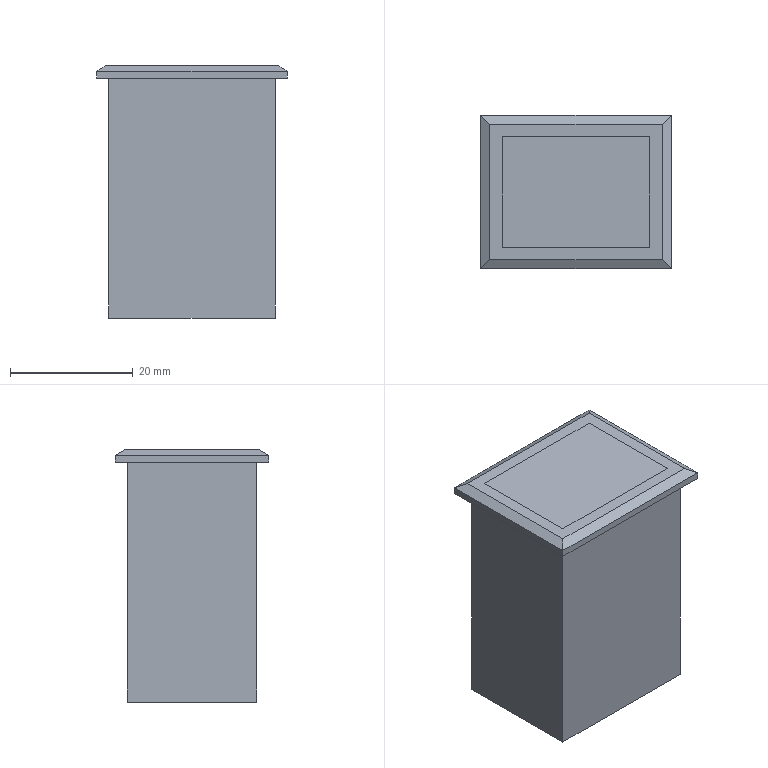Part | SolidWorks | features Chamfer 1, Extrusion 1, ICE 1, PLine 1 | 1 solid | 16 faces | box 31 x 25 x 41 mm | volume 23593 mm3 | plane 16
STEP:
#1=CARTESIAN_POINT('',(-14.,11.,41.));
#2=VERTEX_POINT('',#1);
#3=CARTESIAN_POINT('',(-14.,-11.,41.));
#4=VERTEX_POINT('',#3);
#5=CARTESIAN_POINT('',(-14.,12.5,41.));
#6=DIRECTION('',(0.,-1.,0.));
#7=VECTOR('',#6,1000.);
#8=LINE('',#5,#7);
#9=EDGE_CURVE('',#2,#4,#8,.T.);
#10=ORIENTED_EDGE('',*,*,#9,.T.);
#11=CARTESIAN_POINT('',(14.,-11.,41.));
#12=VERTEX_POINT('',#11);
#13=CARTESIAN_POINT('',(15.5,-11.,41.));
#14=DIRECTION('',(1.,0.,0.));
#15=VECTOR('',#14,1000.);
#16=LINE('',#13,#15);
#17=EDGE_CURVE('',#4,#12,#16,.T.);
#18=ORIENTED_EDGE('',*,*,#17,.T.);
#19=CARTESIAN_POINT('',(14.,11.,41.));
#20=VERTEX_POINT('',#19);
#21=CARTESIAN_POINT('',(14.,12.5,41.));
#22=DIRECTION('',(0.,1.,0.));
#23=VECTOR('',#22,1000.);
#24=LINE('',#21,#23);
#25=EDGE_CURVE('',#12,#20,#24,.T.);
#26=ORIENTED_EDGE('',*,*,#25,.T.);
#27=CARTESIAN_POINT('',(15.5,11.,41.));
#28=DIRECTION('',(-1.,0.,0.));
#29=VECTOR('',#28,1000.);
#30=LINE('',#27,#29);
#31=EDGE_CURVE('',#20,#2,#30,.T.);
#32=ORIENTED_EDGE('',*,*,#31,.T.);
#33=EDGE_LOOP('',(#10,#18,#26,#32));
#34=FACE_OUTER_BOUND('',#33,.T.);
#35=CARTESIAN_POINT('',(12.,-9.,41.));
#36=VERTEX_POINT('',#35);
#37=CARTESIAN_POINT('',(12.,9.,41.));
#38=VERTEX_POINT('',#37);
#39=CARTESIAN_POINT('',(12.,12.5,41.));
#40=DIRECTION('',(0.,1.,0.));
#41=VECTOR('',#40,1000.);
#42=LINE('',#39,#41);
#43=EDGE_CURVE('',#36,#38,#42,.T.);
#44=ORIENTED_EDGE('',*,*,#43,.F.);
#45=CARTESIAN_POINT('',(-12.,-9.,41.));
#46=VERTEX_POINT('',#45);
#47=CARTESIAN_POINT('',(15.5,-9.,41.));
#48=DIRECTION('',(1.,0.,0.));
#49=VECTOR('',#48,1000.);
#50=LINE('',#47,#49);
#51=EDGE_CURVE('',#46,#36,#50,.T.);
#52=ORIENTED_EDGE('',*,*,#51,.F.);
#53=CARTESIAN_POINT('',(-12.,9.,41.));
#54=VERTEX_POINT('',#53);
#55=CARTESIAN_POINT('',(-12.,12.5,41.));
#56=DIRECTION('',(0.,-1.,0.));
#57=VECTOR('',#56,1000.);
#58=LINE('',#55,#57);
#59=EDGE_CURVE('',#54,#46,#58,.T.);
#60=ORIENTED_EDGE('',*,*,#59,.F.);
#61=CARTESIAN_POINT('',(15.5,9.,41.));
#62=DIRECTION('',(-1.,0.,0.));
#63=VECTOR('',#62,1000.);
#64=LINE('',#61,#63);
#65=EDGE_CURVE('',#38,#54,#64,.T.);
#66=ORIENTED_EDGE('',*,*,#65,.F.);
#67=EDGE_LOOP('',(#44,#52,#60,#66));
#68=FACE_BOUND('',#67,.T.);
#69=CARTESIAN_POINT('',(15.5,12.5,41.));
#70=DIRECTION('',(0.,0.,-1.));
#71=DIRECTION('',(-1.,0.,0.));
#72=AXIS2_PLACEMENT_3D('',#69,#70,#71);
#73=PLANE('',#72);
#74=ADVANCED_FACE('',(#34,#68),#73,.F.);
#75=CARTESIAN_POINT('',(13.5,-10.5,0.));
#76=VERTEX_POINT('',#75);
#77=CARTESIAN_POINT('',(13.5,10.5,0.));
#78=VERTEX_POINT('',#77);
#79=CARTESIAN_POINT('',(13.5,-10.5,0.));
#80=DIRECTION('',(0.,1.,0.));
#81=VECTOR('',#80,1000.);
#82=LINE('',#79,#81);
#83=EDGE_CURVE('',#76,#78,#82,.T.);
#84=ORIENTED_EDGE('',*,*,#83,.T.);
#85=CARTESIAN_POINT('',(13.5,10.5,39.));
#86=VERTEX_POINT('',#85);
#87=CARTESIAN_POINT('',(13.5,10.5,39.));
#88=DIRECTION('',(0.,0.,-1.));
#89=VECTOR('',#88,1000.);
#90=LINE('',#87,#89);
#91=EDGE_CURVE('',#86,#78,#90,.T.);
#92=ORIENTED_EDGE('',*,*,#91,.F.);
#93=CARTESIAN_POINT('',(13.5,-10.5,39.));
#94=VERTEX_POINT('',#93);
#95=CARTESIAN_POINT('',(13.5,-10.5,39.));
#96=DIRECTION('',(0.,1.,0.));
#97=VECTOR('',#96,1000.);
#98=LINE('',#95,#97);
#99=EDGE_CURVE('',#94,#86,#98,.T.);
#100=ORIENTED_EDGE('',*,*,#99,.F.);
#101=CARTESIAN_POINT('',(13.5,-10.5,39.));
#102=DIRECTION('',(0.,0.,-1.));
#103=VECTOR('',#102,1000.);
#104=LINE('',#101,#103);
#105=EDGE_CURVE('',#94,#76,#104,.T.);
#106=ORIENTED_EDGE('',*,*,#105,.T.);
#107=EDGE_LOOP('',(#84,#92,#100,#106));
#108=FACE_OUTER_BOUND('',#107,.T.);
#109=CARTESIAN_POINT('',(13.5,-10.5,39.));
#110=DIRECTION('',(-1.,0.,0.));
#111=DIRECTION('',(0.,0.,1.));
#112=AXIS2_PLACEMENT_3D('',#109,#110,#111);
#113=PLANE('',#112);
#114=ADVANCED_FACE('',(#108),#113,.F.);
#115=CARTESIAN_POINT('',(-13.5,10.5,0.));
#116=VERTEX_POINT('',#115);
#117=CARTESIAN_POINT('',(-13.5,10.5,0.));
#118=DIRECTION('',(-1.,0.,0.));
#119=VECTOR('',#118,1000.);
#120=LINE('',#117,#119);
#121=EDGE_CURVE('',#78,#116,#120,.T.);
#122=ORIENTED_EDGE('',*,*,#121,.T.);
#123=CARTESIAN_POINT('',(-13.5,10.5,39.));
#124=VERTEX_POINT('',#123);
#125=CARTESIAN_POINT('',(-13.5,10.5,39.));
#126=DIRECTION('',(0.,0.,-1.));
#127=VECTOR('',#126,1000.);
#128=LINE('',#125,#127);
#129=EDGE_CURVE('',#124,#116,#128,.T.);
#130=ORIENTED_EDGE('',*,*,#129,.F.);
#131=CARTESIAN_POINT('',(-13.5,10.5,39.));
#132=DIRECTION('',(-1.,0.,0.));
#133=VECTOR('',#132,1000.);
#134=LINE('',#131,#133);
#135=EDGE_CURVE('',#86,#124,#134,.T.);
#136=ORIENTED_EDGE('',*,*,#135,.F.);
#137=ORIENTED_EDGE('',*,*,#91,.T.);
#138=EDGE_LOOP('',(#122,#130,#136,#137));
#139=FACE_OUTER_BOUND('',#138,.T.);
#140=CARTESIAN_POINT('',(-13.5,10.5,39.));
#141=DIRECTION('',(0.,-1.,0.));
#142=DIRECTION('',(0.,0.,-1.));
#143=AXIS2_PLACEMENT_3D('',#140,#141,#142);
#144=PLANE('',#143);
#145=ADVANCED_FACE('',(#139),#144,.F.);
#146=CARTESIAN_POINT('',(-13.5,-10.5,0.));
#147=VERTEX_POINT('',#146);
#148=CARTESIAN_POINT('',(-13.5,-10.5,0.));
#149=DIRECTION('',(0.,-1.,0.));
#150=VECTOR('',#149,1000.);
#151=LINE('',#148,#150);
#152=EDGE_CURVE('',#116,#147,#151,.T.);
#153=ORIENTED_EDGE('',*,*,#152,.T.);
#154=CARTESIAN_POINT('',(-13.5,-10.5,39.));
#155=VERTEX_POINT('',#154);
#156=CARTESIAN_POINT('',(-13.5,-10.5,39.));
#157=DIRECTION('',(0.,0.,-1.));
#158=VECTOR('',#157,1000.);
#159=LINE('',#156,#158);
#160=EDGE_CURVE('',#155,#147,#159,.T.);
#161=ORIENTED_EDGE('',*,*,#160,.F.);
#162=CARTESIAN_POINT('',(-13.5,-10.5,39.));
#163=DIRECTION('',(0.,-1.,0.));
#164=VECTOR('',#163,1000.);
#165=LINE('',#162,#164);
#166=EDGE_CURVE('',#124,#155,#165,.T.);
#167=ORIENTED_EDGE('',*,*,#166,.F.);
#168=ORIENTED_EDGE('',*,*,#129,.T.);
#169=EDGE_LOOP('',(#153,#161,#167,#168));
#170=FACE_OUTER_BOUND('',#169,.T.);
#171=CARTESIAN_POINT('',(-13.5,-10.5,39.));
#172=DIRECTION('',(1.,0.,0.));
#173=DIRECTION('',(0.,0.,-1.));
#174=AXIS2_PLACEMENT_3D('',#171,#172,#173);
#175=PLANE('',#174);
#176=ADVANCED_FACE('',(#170),#175,.F.);
#177=CARTESIAN_POINT('',(-13.5,-10.5,0.));
#178=DIRECTION('',(1.,0.,0.));
#179=VECTOR('',#178,1000.);
#180=LINE('',#177,#179);
#181=EDGE_CURVE('',#147,#76,#180,.T.);
#182=ORIENTED_EDGE('',*,*,#181,.T.);
#183=ORIENTED_EDGE('',*,*,#105,.F.);
#184=CARTESIAN_POINT('',(-13.5,-10.5,39.));
#185=DIRECTION('',(1.,0.,0.));
#186=VECTOR('',#185,1000.);
#187=LINE('',#184,#186);
#188=EDGE_CURVE('',#155,#94,#187,.T.);
#189=ORIENTED_EDGE('',*,*,#188,.F.);
#190=ORIENTED_EDGE('',*,*,#160,.T.);
#191=EDGE_LOOP('',(#182,#183,#189,#190));
#192=FACE_OUTER_BOUND('',#191,.T.);
#193=CARTESIAN_POINT('',(-13.5,-10.5,39.));
#194=DIRECTION('',(0.,1.,0.));
#195=DIRECTION('',(0.,0.,1.));
#196=AXIS2_PLACEMENT_3D('',#193,#194,#195);
#197=PLANE('',#196);
#198=ADVANCED_FACE('',(#192),#197,.F.);
#199=ORIENTED_EDGE('',*,*,#83,.F.);
#200=ORIENTED_EDGE('',*,*,#181,.F.);
#201=ORIENTED_EDGE('',*,*,#152,.F.);
#202=ORIENTED_EDGE('',*,*,#121,.F.);
#203=EDGE_LOOP('',(#199,#200,#201,#202));
#204=FACE_OUTER_BOUND('',#203,.T.);
#205=CARTESIAN_POINT('',(13.5,10.5,0.));
#206=DIRECTION('',(0.,0.,-1.));
#207=DIRECTION('',(-1.,0.,0.));
#208=AXIS2_PLACEMENT_3D('',#205,#206,#207);
#209=PLANE('',#208);
#210=ADVANCED_FACE('',(#204),#209,.T.);
#211=CARTESIAN_POINT('',(15.5,-12.5,39.));
#212=VERTEX_POINT('',#211);
#213=CARTESIAN_POINT('',(15.5,12.5,39.));
#214=VERTEX_POINT('',#213);
#215=CARTESIAN_POINT('',(15.5,-12.5,39.));
#216=DIRECTION('',(0.,1.,0.));
#217=VECTOR('',#216,1000.);
#218=LINE('',#215,#217);
#219=EDGE_CURVE('',#212,#214,#218,.T.);
#220=ORIENTED_EDGE('',*,*,#219,.F.);
#221=CARTESIAN_POINT('',(-15.5,-12.5,39.));
#222=VERTEX_POINT('',#221);
#223=CARTESIAN_POINT('',(-15.5,-12.5,39.));
#224=DIRECTION('',(1.,0.,0.));
#225=VECTOR('',#224,1000.);
#226=LINE('',#223,#225);
#227=EDGE_CURVE('',#222,#212,#226,.T.);
#228=ORIENTED_EDGE('',*,*,#227,.F.);
#229=CARTESIAN_POINT('',(-15.5,12.5,39.));
#230=VERTEX_POINT('',#229);
#231=CARTESIAN_POINT('',(-15.5,-12.5,39.));
#232=DIRECTION('',(0.,-1.,0.));
#233=VECTOR('',#232,1000.);
#234=LINE('',#231,#233);
#235=EDGE_CURVE('',#230,#222,#234,.T.);
#236=ORIENTED_EDGE('',*,*,#235,.F.);
#237=CARTESIAN_POINT('',(-15.5,12.5,39.));
#238=DIRECTION('',(-1.,0.,0.));
#239=VECTOR('',#238,1000.);
#240=LINE('',#237,#239);
#241=EDGE_CURVE('',#214,#230,#240,.T.);
#242=ORIENTED_EDGE('',*,*,#241,.F.);
#243=EDGE_LOOP('',(#220,#228,#236,#242));
#244=FACE_OUTER_BOUND('',#243,.T.);
#245=ORIENTED_EDGE('',*,*,#99,.T.);
#246=ORIENTED_EDGE('',*,*,#135,.T.);
#247=ORIENTED_EDGE('',*,*,#166,.T.);
#248=ORIENTED_EDGE('',*,*,#188,.T.);
#249=EDGE_LOOP('',(#245,#246,#247,#248));
#250=FACE_BOUND('',#249,.T.);
#251=CARTESIAN_POINT('',(15.5,12.5,39.));
#252=DIRECTION('',(0.,0.,-1.));
#253=DIRECTION('',(-1.,0.,0.));
#254=AXIS2_PLACEMENT_3D('',#251,#252,#253);
#255=PLANE('',#254);
#256=ADVANCED_FACE('',(#244,#250),#255,.T.);
#257=CARTESIAN_POINT('',(15.5,12.5,40.134));
#258=VERTEX_POINT('',#257);
#259=CARTESIAN_POINT('',(15.5,12.5,41.));
#260=DIRECTION('',(0.,0.,-1.));
#261=VECTOR('',#260,1000.);
#262=LINE('',#259,#261);
#263=EDGE_CURVE('',#258,#214,#262,.T.);
#264=ORIENTED_EDGE('',*,*,#263,.F.);
#265=CARTESIAN_POINT('',(15.5,-12.5,40.134));
#266=VERTEX_POINT('',#265);
#267=CARTESIAN_POINT('',(15.5,-12.5,40.134));
#268=DIRECTION('',(0.,-1.,0.));
#269=VECTOR('',#268,1000.);
#270=LINE('',#267,#269);
#271=EDGE_CURVE('',#258,#266,#270,.T.);
#272=ORIENTED_EDGE('',*,*,#271,.T.);
#273=CARTESIAN_POINT('',(15.5,-12.5,41.));
#274=DIRECTION('',(0.,0.,-1.));
#275=VECTOR('',#274,1000.);
#276=LINE('',#273,#275);
#277=EDGE_CURVE('',#266,#212,#276,.T.);
#278=ORIENTED_EDGE('',*,*,#277,.T.);
#279=ORIENTED_EDGE('',*,*,#219,.T.);
#280=EDGE_LOOP('',(#264,#272,#278,#279));
#281=FACE_OUTER_BOUND('',#280,.T.);
#282=CARTESIAN_POINT('',(15.5,-12.5,41.));
#283=DIRECTION('',(-1.,0.,0.));
#284=DIRECTION('',(0.,0.,1.));
#285=AXIS2_PLACEMENT_3D('',#282,#283,#284);
#286=PLANE('',#285);
#287=ADVANCED_FACE('',(#281),#286,.F.);
#288=CARTESIAN_POINT('',(-15.5,12.5,40.134));
#289=VERTEX_POINT('',#288);
#290=CARTESIAN_POINT('',(-15.5,12.5,41.));
#291=DIRECTION('',(0.,0.,-1.));
#292=VECTOR('',#291,1000.);
#293=LINE('',#290,#292);
#294=EDGE_CURVE('',#289,#230,#293,.T.);
#295=ORIENTED_EDGE('',*,*,#294,.F.);
#296=CARTESIAN_POINT('',(-15.5,12.5,40.134));
#297=DIRECTION('',(1.,0.,0.));
#298=VECTOR('',#297,1000.);
#299=LINE('',#296,#298);
#300=EDGE_CURVE('',#289,#258,#299,.T.);
#301=ORIENTED_EDGE('',*,*,#300,.T.);
#302=ORIENTED_EDGE('',*,*,#263,.T.);
#303=ORIENTED_EDGE('',*,*,#241,.T.);
#304=EDGE_LOOP('',(#295,#301,#302,#303));
#305=FACE_OUTER_BOUND('',#304,.T.);
#306=CARTESIAN_POINT('',(-15.5,12.5,41.));
#307=DIRECTION('',(0.,-1.,0.));
#308=DIRECTION('',(0.,0.,-1.));
#309=AXIS2_PLACEMENT_3D('',#306,#307,#308);
#310=PLANE('',#309);
#311=ADVANCED_FACE('',(#305),#310,.F.);
#312=CARTESIAN_POINT('',(-15.5,-12.5,40.134));
#313=VERTEX_POINT('',#312);
#314=CARTESIAN_POINT('',(-15.5,-12.5,41.));
#315=DIRECTION('',(0.,0.,-1.));
#316=VECTOR('',#315,1000.);
#317=LINE('',#314,#316);
#318=EDGE_CURVE('',#313,#222,#317,.T.);
#319=ORIENTED_EDGE('',*,*,#318,.F.);
#320=CARTESIAN_POINT('',(-15.5,-12.5,40.134));
#321=DIRECTION('',(0.,1.,0.));
#322=VECTOR('',#321,1000.);
#323=LINE('',#320,#322);
#324=EDGE_CURVE('',#313,#289,#323,.T.);
#325=ORIENTED_EDGE('',*,*,#324,.T.);
#326=ORIENTED_EDGE('',*,*,#294,.T.);
#327=ORIENTED_EDGE('',*,*,#235,.T.);
#328=EDGE_LOOP('',(#319,#325,#326,#327));
#329=FACE_OUTER_BOUND('',#328,.T.);
#330=CARTESIAN_POINT('',(-15.5,-12.5,41.));
#331=DIRECTION('',(1.,0.,0.));
#332=DIRECTION('',(0.,0.,-1.));
#333=AXIS2_PLACEMENT_3D('',#330,#331,#332);
#334=PLANE('',#333);
#335=ADVANCED_FACE('',(#329),#334,.F.);
#336=ORIENTED_EDGE('',*,*,#277,.F.);
#337=CARTESIAN_POINT('',(-15.5,-12.5,40.134));
#338=DIRECTION('',(-1.,0.,0.));
#339=VECTOR('',#338,1000.);
#340=LINE('',#337,#339);
#341=EDGE_CURVE('',#266,#313,#340,.T.);
#342=ORIENTED_EDGE('',*,*,#341,.T.);
#343=ORIENTED_EDGE('',*,*,#318,.T.);
#344=ORIENTED_EDGE('',*,*,#227,.T.);
#345=EDGE_LOOP('',(#336,#342,#343,#344));
#346=FACE_OUTER_BOUND('',#345,.T.);
#347=CARTESIAN_POINT('',(-15.5,-12.5,41.));
#348=DIRECTION('',(0.,1.,0.));
#349=DIRECTION('',(0.,0.,1.));
#350=AXIS2_PLACEMENT_3D('',#347,#348,#349);
#351=PLANE('',#350);
#352=ADVANCED_FACE('',(#346),#351,.F.);
#353=ORIENTED_EDGE('',*,*,#51,.T.);
#354=ORIENTED_EDGE('',*,*,#43,.T.);
#355=ORIENTED_EDGE('',*,*,#65,.T.);
#356=ORIENTED_EDGE('',*,*,#59,.T.);
#357=EDGE_LOOP('',(#353,#354,#355,#356));
#358=FACE_OUTER_BOUND('',#357,.T.);
#359=CARTESIAN_POINT('',(15.5,12.5,41.));
#360=DIRECTION('',(0.,0.,-1.));
#361=DIRECTION('',(-1.,0.,0.));
#362=AXIS2_PLACEMENT_3D('',#359,#360,#361);
#363=PLANE('',#362);
#364=ADVANCED_FACE('',(#358),#363,.F.);
#365=CARTESIAN_POINT('',(14.643,11.643,40.629));
#366=DIRECTION('',(-0.6547,-0.6547,0.378));
#367=VECTOR('',#366,1000.);
#368=LINE('',#365,#367);
#369=EDGE_CURVE('',#258,#20,#368,.T.);
#370=ORIENTED_EDGE('',*,*,#369,.F.);
#371=ORIENTED_EDGE('',*,*,#300,.F.);
#372=CARTESIAN_POINT('',(-1.357,-1.643,48.299));
#373=DIRECTION('',(-0.6547,0.6547,-0.378));
#374=VECTOR('',#373,1000.);
#375=LINE('',#372,#374);
#376=EDGE_CURVE('',#2,#289,#375,.T.);
#377=ORIENTED_EDGE('',*,*,#376,.F.);
#378=ORIENTED_EDGE('',*,*,#31,.F.);
#379=EDGE_LOOP('',(#370,#371,#377,#378));
#380=FACE_OUTER_BOUND('',#379,.T.);
#381=CARTESIAN_POINT('',(15.5,11.,41.));
#382=DIRECTION('',(0.,-0.5,-0.866));
#383=DIRECTION('',(-1.,0.,0.));
#384=AXIS2_PLACEMENT_3D('',#381,#382,#383);
#385=PLANE('',#384);
#386=ADVANCED_FACE('',(#380),#385,.F.);
#387=ORIENTED_EDGE('',*,*,#376,.T.);
#388=ORIENTED_EDGE('',*,*,#324,.F.);
#389=CARTESIAN_POINT('',(-3.929,-0.9286,46.815));
#390=DIRECTION('',(-0.6547,-0.6547,-0.378));
#391=VECTOR('',#390,1000.);
#392=LINE('',#389,#391);
#393=EDGE_CURVE('',#4,#313,#392,.T.);
#394=ORIENTED_EDGE('',*,*,#393,.F.);
#395=ORIENTED_EDGE('',*,*,#9,.F.);
#396=EDGE_LOOP('',(#387,#388,#394,#395));
#397=FACE_OUTER_BOUND('',#396,.T.);
#398=CARTESIAN_POINT('',(-14.,12.5,41.));
#399=DIRECTION('',(0.5,0.,-0.866));
#400=DIRECTION('',(0.,-1.,0.));
#401=AXIS2_PLACEMENT_3D('',#398,#399,#400);
#402=PLANE('',#401);
#403=ADVANCED_FACE('',(#397),#402,.F.);
#404=ORIENTED_EDGE('',*,*,#369,.T.);
#405=ORIENTED_EDGE('',*,*,#25,.F.);
#406=CARTESIAN_POINT('',(3.929,-0.9286,46.815));
#407=DIRECTION('',(-0.6547,0.6547,0.378));
#408=VECTOR('',#407,1000.);
#409=LINE('',#406,#408);
#410=EDGE_CURVE('',#266,#12,#409,.T.);
#411=ORIENTED_EDGE('',*,*,#410,.F.);
#412=ORIENTED_EDGE('',*,*,#271,.F.);
#413=EDGE_LOOP('',(#404,#405,#411,#412));
#414=FACE_OUTER_BOUND('',#413,.T.);
#415=CARTESIAN_POINT('',(14.,12.5,41.));
#416=DIRECTION('',(-0.5,0.,-0.866));
#417=DIRECTION('',(0.,1.,0.));
#418=AXIS2_PLACEMENT_3D('',#415,#416,#417);
#419=PLANE('',#418);
#420=ADVANCED_FACE('',(#414),#419,.F.);
#421=ORIENTED_EDGE('',*,*,#393,.T.);
#422=ORIENTED_EDGE('',*,*,#341,.F.);
#423=ORIENTED_EDGE('',*,*,#410,.T.);
#424=ORIENTED_EDGE('',*,*,#17,.F.);
#425=EDGE_LOOP('',(#421,#422,#423,#424));
#426=FACE_OUTER_BOUND('',#425,.T.);
#427=CARTESIAN_POINT('',(15.5,-11.,41.));
#428=DIRECTION('',(0.,0.5,-0.866));
#429=DIRECTION('',(1.,0.,0.));
#430=AXIS2_PLACEMENT_3D('',#427,#428,#429);
#431=PLANE('',#430);
#432=ADVANCED_FACE('',(#426),#431,.F.);
#433=CLOSED_SHELL('',(#74,#114,#145,#176,#198,#210,#256,#287,#311,#335,#352,#364,#386,#403,#420,#432));
#434=MANIFOLD_SOLID_BREP('',#433);
#435=CARTESIAN_POINT('',(0.,0.,0.));
#436=DIRECTION('',(0.,0.,1.));
#437=DIRECTION('',(1.,0.,0.));
#438=AXIS2_PLACEMENT_3D('',#435,#436,#437);
#439=(LENGTH_UNIT()NAMED_UNIT(*)SI_UNIT(.MILLI.,.METRE.));
#440=UNCERTAINTY_MEASURE_WITH_UNIT(LENGTH_MEASURE(0.00001),#439,'','');
#441=(NAMED_UNIT(*)PLANE_ANGLE_UNIT()SI_UNIT($,.RADIAN.));
#442=(NAMED_UNIT(*)SI_UNIT($,.STERADIAN.)SOLID_ANGLE_UNIT());
#443=(GEOMETRIC_REPRESENTATION_CONTEXT(3)GLOBAL_UNCERTAINTY_ASSIGNED_CONTEXT((#440))GLOBAL_UNIT_ASSIGNED_CONTEXT((#439,#441,#442))REPRESENTATION_CONTEXT('',''));
#444=ADVANCED_BREP_SHAPE_REPRESENTATION('',(#434,#438),#443);